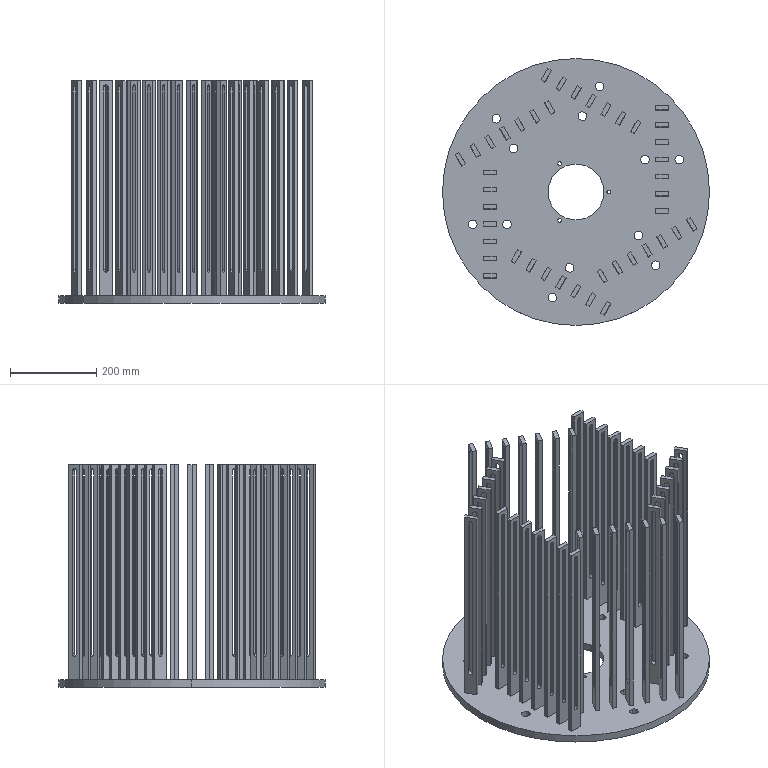Part | Creo | features CUT 12, PROTRUSION 7, CURVE 4, DATUM PLANE 3, PATTERN 3, COORDINATE SYSTEM 1 | 1 solid | 449 faces | box 620 x 620 x 518 mm | volume 9371630 mm3 | plane 331 | cylinder 118 | commonest cylinder face diameters 10.5 x84 20 x24 8.5 x6 130 x2 620 x2